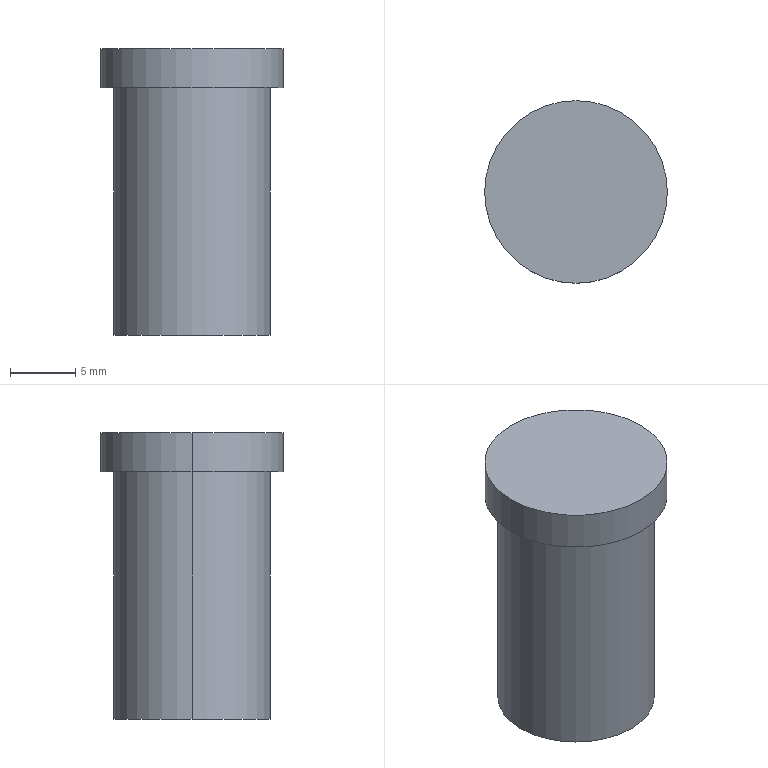Part | SolidWorks | features Revolution 1 | 1 solid | 7 faces | box 14 x 14 x 22 mm | volume 2611 mm3 | cylinder 4 | plane 3 | commonest cylinder face diameters 12 x2 14 x2
STEP:
#1=CARTESIAN_POINT('',(-6.,0.,-3.));
#2=VERTEX_POINT('',#1);
#3=CARTESIAN_POINT('',(6.,0.,-3.));
#4=VERTEX_POINT('',#3);
#5=CARTESIAN_POINT('',(0.,0.,-3.));
#6=DIRECTION('',(0.,0.,-1.));
#7=DIRECTION('',(-1.,0.,0.));
#8=AXIS2_PLACEMENT_3D('',#5,#6,#7);
#9=CIRCLE('',#8,6.);
#10=EDGE_CURVE('',#2,#4,#9,.T.);
#11=ORIENTED_EDGE('',*,*,#10,.T.);
#12=CARTESIAN_POINT('',(6.,0.,-22.));
#13=VERTEX_POINT('',#12);
#14=CARTESIAN_POINT('',(6.,0.,-22.));
#15=DIRECTION('',(0.,0.,-1.));
#16=VECTOR('',#15,1000.);
#17=LINE('',#14,#16);
#18=EDGE_CURVE('',#4,#13,#17,.T.);
#19=ORIENTED_EDGE('',*,*,#18,.T.);
#20=CARTESIAN_POINT('',(-6.,0.,-22.));
#21=VERTEX_POINT('',#20);
#22=CARTESIAN_POINT('',(0.,0.,-22.));
#23=DIRECTION('',(0.,0.,-1.));
#24=DIRECTION('',(-1.,0.,0.));
#25=AXIS2_PLACEMENT_3D('',#22,#23,#24);
#26=CIRCLE('',#25,6.);
#27=EDGE_CURVE('',#21,#13,#26,.T.);
#28=ORIENTED_EDGE('',*,*,#27,.F.);
#29=CARTESIAN_POINT('',(-6.,0.,-22.));
#30=DIRECTION('',(0.,0.,-1.));
#31=VECTOR('',#30,1000.);
#32=LINE('',#29,#31);
#33=EDGE_CURVE('',#2,#21,#32,.T.);
#34=ORIENTED_EDGE('',*,*,#33,.F.);
#35=EDGE_LOOP('',(#11,#19,#28,#34));
#36=FACE_OUTER_BOUND('',#35,.T.);
#37=CARTESIAN_POINT('',(0.,0.,-22.));
#38=DIRECTION('',(0.,0.,-1.));
#39=DIRECTION('',(-1.,0.,0.));
#40=AXIS2_PLACEMENT_3D('',#37,#38,#39);
#41=CYLINDRICAL_SURFACE('',#40,6.);
#42=ADVANCED_FACE('',(#36),#41,.T.);
#43=CARTESIAN_POINT('',(-7.,0.,0.));
#44=VERTEX_POINT('',#43);
#45=CARTESIAN_POINT('',(7.,0.,0.));
#46=VERTEX_POINT('',#45);
#47=CARTESIAN_POINT('',(0.,0.,0.));
#48=DIRECTION('',(0.,0.,-1.));
#49=DIRECTION('',(-1.,0.,0.));
#50=AXIS2_PLACEMENT_3D('',#47,#48,#49);
#51=CIRCLE('',#50,7.);
#52=EDGE_CURVE('',#44,#46,#51,.T.);
#53=ORIENTED_EDGE('',*,*,#52,.T.);
#54=CARTESIAN_POINT('',(7.,0.,-3.));
#55=VERTEX_POINT('',#54);
#56=CARTESIAN_POINT('',(7.,0.,-22.));
#57=DIRECTION('',(0.,0.,-1.));
#58=VECTOR('',#57,1000.);
#59=LINE('',#56,#58);
#60=EDGE_CURVE('',#46,#55,#59,.T.);
#61=ORIENTED_EDGE('',*,*,#60,.T.);
#62=CARTESIAN_POINT('',(-7.,0.,-3.));
#63=VERTEX_POINT('',#62);
#64=CARTESIAN_POINT('',(0.,0.,-3.));
#65=DIRECTION('',(0.,0.,-1.));
#66=DIRECTION('',(-1.,0.,0.));
#67=AXIS2_PLACEMENT_3D('',#64,#65,#66);
#68=CIRCLE('',#67,7.);
#69=EDGE_CURVE('',#63,#55,#68,.T.);
#70=ORIENTED_EDGE('',*,*,#69,.F.);
#71=CARTESIAN_POINT('',(-7.,0.,-22.));
#72=DIRECTION('',(0.,0.,-1.));
#73=VECTOR('',#72,1000.);
#74=LINE('',#71,#73);
#75=EDGE_CURVE('',#44,#63,#74,.T.);
#76=ORIENTED_EDGE('',*,*,#75,.F.);
#77=EDGE_LOOP('',(#53,#61,#70,#76));
#78=FACE_OUTER_BOUND('',#77,.T.);
#79=CARTESIAN_POINT('',(0.,0.,-22.));
#80=DIRECTION('',(0.,0.,-1.));
#81=DIRECTION('',(-1.,0.,0.));
#82=AXIS2_PLACEMENT_3D('',#79,#80,#81);
#83=CYLINDRICAL_SURFACE('',#82,7.);
#84=ADVANCED_FACE('',(#78),#83,.T.);
#85=ORIENTED_EDGE('',*,*,#52,.F.);
#86=CARTESIAN_POINT('',(0.,0.,0.));
#87=DIRECTION('',(0.,0.,-1.));
#88=DIRECTION('',(-1.,0.,0.));
#89=AXIS2_PLACEMENT_3D('',#86,#87,#88);
#90=CIRCLE('',#89,7.);
#91=EDGE_CURVE('',#46,#44,#90,.T.);
#92=ORIENTED_EDGE('',*,*,#91,.F.);
#93=EDGE_LOOP('',(#85,#92));
#94=FACE_OUTER_BOUND('',#93,.T.);
#95=CARTESIAN_POINT('',(0.,0.,0.));
#96=DIRECTION('',(0.,0.,-1.));
#97=DIRECTION('',(-1.,0.,0.));
#98=AXIS2_PLACEMENT_3D('',#95,#96,#97);
#99=PLANE('',#98);
#100=ADVANCED_FACE('',(#94),#99,.F.);
#101=ORIENTED_EDGE('',*,*,#60,.F.);
#102=ORIENTED_EDGE('',*,*,#91,.T.);
#103=ORIENTED_EDGE('',*,*,#75,.T.);
#104=CARTESIAN_POINT('',(0.,0.,-3.));
#105=DIRECTION('',(0.,0.,-1.));
#106=DIRECTION('',(-1.,0.,0.));
#107=AXIS2_PLACEMENT_3D('',#104,#105,#106);
#108=CIRCLE('',#107,7.);
#109=EDGE_CURVE('',#55,#63,#108,.T.);
#110=ORIENTED_EDGE('',*,*,#109,.F.);
#111=EDGE_LOOP('',(#101,#102,#103,#110));
#112=FACE_OUTER_BOUND('',#111,.T.);
#113=CARTESIAN_POINT('',(0.,0.,-22.));
#114=DIRECTION('',(0.,0.,-1.));
#115=DIRECTION('',(-1.,0.,0.));
#116=AXIS2_PLACEMENT_3D('',#113,#114,#115);
#117=CYLINDRICAL_SURFACE('',#116,7.);
#118=ADVANCED_FACE('',(#112),#117,.T.);
#119=ORIENTED_EDGE('',*,*,#10,.F.);
#120=CARTESIAN_POINT('',(0.,0.,-3.));
#121=DIRECTION('',(0.,0.,-1.));
#122=DIRECTION('',(-1.,0.,0.));
#123=AXIS2_PLACEMENT_3D('',#120,#121,#122);
#124=CIRCLE('',#123,6.);
#125=EDGE_CURVE('',#4,#2,#124,.T.);
#126=ORIENTED_EDGE('',*,*,#125,.F.);
#127=EDGE_LOOP('',(#119,#126));
#128=FACE_BOUND('',#127,.T.);
#129=ORIENTED_EDGE('',*,*,#69,.T.);
#130=ORIENTED_EDGE('',*,*,#109,.T.);
#131=EDGE_LOOP('',(#129,#130));
#132=FACE_OUTER_BOUND('',#131,.T.);
#133=CARTESIAN_POINT('',(7.,0.,-3.));
#134=DIRECTION('',(0.,0.,1.));
#135=DIRECTION('',(1.,0.,0.));
#136=AXIS2_PLACEMENT_3D('',#133,#134,#135);
#137=PLANE('',#136);
#138=ADVANCED_FACE('',(#128,#132),#137,.F.);
#139=ORIENTED_EDGE('',*,*,#18,.F.);
#140=ORIENTED_EDGE('',*,*,#125,.T.);
#141=ORIENTED_EDGE('',*,*,#33,.T.);
#142=CARTESIAN_POINT('',(0.,0.,-22.));
#143=DIRECTION('',(0.,0.,-1.));
#144=DIRECTION('',(-1.,0.,0.));
#145=AXIS2_PLACEMENT_3D('',#142,#143,#144);
#146=CIRCLE('',#145,6.);
#147=EDGE_CURVE('',#13,#21,#146,.T.);
#148=ORIENTED_EDGE('',*,*,#147,.F.);
#149=EDGE_LOOP('',(#139,#140,#141,#148));
#150=FACE_OUTER_BOUND('',#149,.T.);
#151=CARTESIAN_POINT('',(0.,0.,-22.));
#152=DIRECTION('',(0.,0.,-1.));
#153=DIRECTION('',(-1.,0.,0.));
#154=AXIS2_PLACEMENT_3D('',#151,#152,#153);
#155=CYLINDRICAL_SURFACE('',#154,6.);
#156=ADVANCED_FACE('',(#150),#155,.T.);
#157=ORIENTED_EDGE('',*,*,#27,.T.);
#158=ORIENTED_EDGE('',*,*,#147,.T.);
#159=EDGE_LOOP('',(#157,#158));
#160=FACE_OUTER_BOUND('',#159,.T.);
#161=CARTESIAN_POINT('',(6.,0.,-22.));
#162=DIRECTION('',(0.,0.,1.));
#163=DIRECTION('',(1.,0.,0.));
#164=AXIS2_PLACEMENT_3D('',#161,#162,#163);
#165=PLANE('',#164);
#166=ADVANCED_FACE('',(#160),#165,.F.);
#167=CLOSED_SHELL('',(#42,#84,#100,#118,#138,#156,#166));
#168=MANIFOLD_SOLID_BREP('',#167);
#169=CARTESIAN_POINT('',(0.,0.,0.));
#170=DIRECTION('',(0.,0.,1.));
#171=DIRECTION('',(1.,0.,0.));
#172=AXIS2_PLACEMENT_3D('',#169,#170,#171);
#173=(LENGTH_UNIT()NAMED_UNIT(*)SI_UNIT(.MILLI.,.METRE.));
#174=UNCERTAINTY_MEASURE_WITH_UNIT(LENGTH_MEASURE(0.00001),#173,'','');
#175=(NAMED_UNIT(*)PLANE_ANGLE_UNIT()SI_UNIT($,.RADIAN.));
#176=(NAMED_UNIT(*)SI_UNIT($,.STERADIAN.)SOLID_ANGLE_UNIT());
#177=(GEOMETRIC_REPRESENTATION_CONTEXT(3)GLOBAL_UNCERTAINTY_ASSIGNED_CONTEXT((#174))GLOBAL_UNIT_ASSIGNED_CONTEXT((#173,#175,#176))REPRESENTATION_CONTEXT('',''));
#178=ADVANCED_BREP_SHAPE_REPRESENTATION('',(#168,#172),#177);